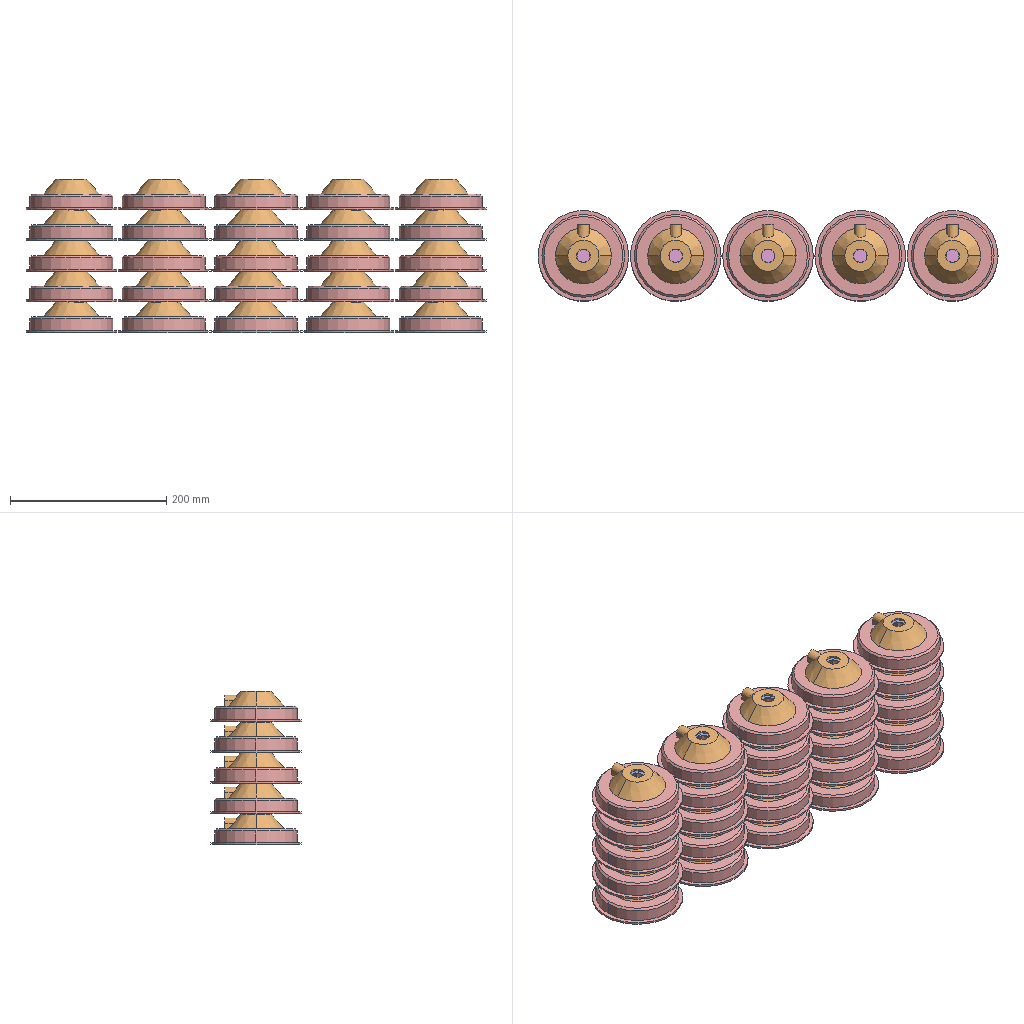Assembly | SolidWorks | 6 different items | 150 placed | box 588 x 115 x 196 mm
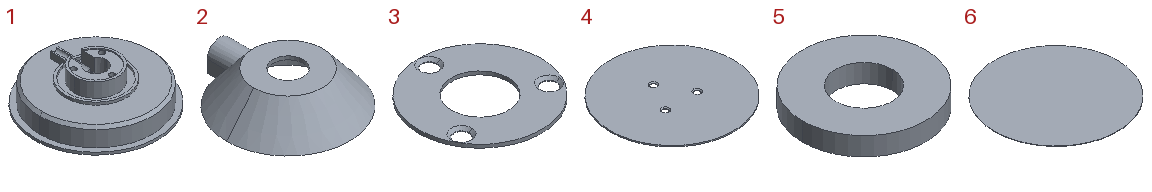Parts list (item | quantity | size | volume | features):
1 | x25 | 116 x 116 x 33.3 mm | 52599 mm3 | features ICE 11, Chamfer 1, Extrusion 1
2 | x25 | 71.8 x 75.9 x 19 mm | 15603 mm3 | features ICE 5, Extrusion 1, RevCut 1
3 | x25 | 36.5 x 36.5 x 1 mm | 761.783 mm3 | features Chamfer 1, Extrusion 1
4 | x25 | 100 x 100 x 1 mm | 7791 mm3 | features Chamfer 1, Extrusion 1
5 | x25 | 100 x 100 x 15 mm | 93420 mm3 | features Extrusion 1
6 | x25 | 108 x 108 x 0.3 mm | 2748 mm3 | features Extrusion 1
Mates (type | each side: item.copy, entity, surface, feature):
Coincident | 1.1 face plane Cut-Extrude 1 | 3.1 face plane Boss-Extrude 1
Coincident | 1.1 plane | 3.1 plane
Concentric | 1.1 edge | 3.1 edge
Coincident | 1.1 face plane Cut-Extrude 3 | 5.1 face plane Boss-Extrude 1
Concentric | 1.1 edge | 5.1 edge
Concentric | 1.1 edge | 4.1 edge
Coincident | 1.1 face plane Boss-Extrude 1 | 6.1 face plane Boss-Extrude 1
Concentric | 1.1 edge | 6.1 edge
Coincident | 1.1 face plane Boss-Extrude 2 | 2.1 face plane Boss-Extrude 1
Concentric | 1.1 edge | 2.1 edge
Coincident | 5.1 face plane Boss-Extrude 1 | 4.1 face plane Boss-Extrude 1
Coincident | 5.1 plane | 4.1 plane